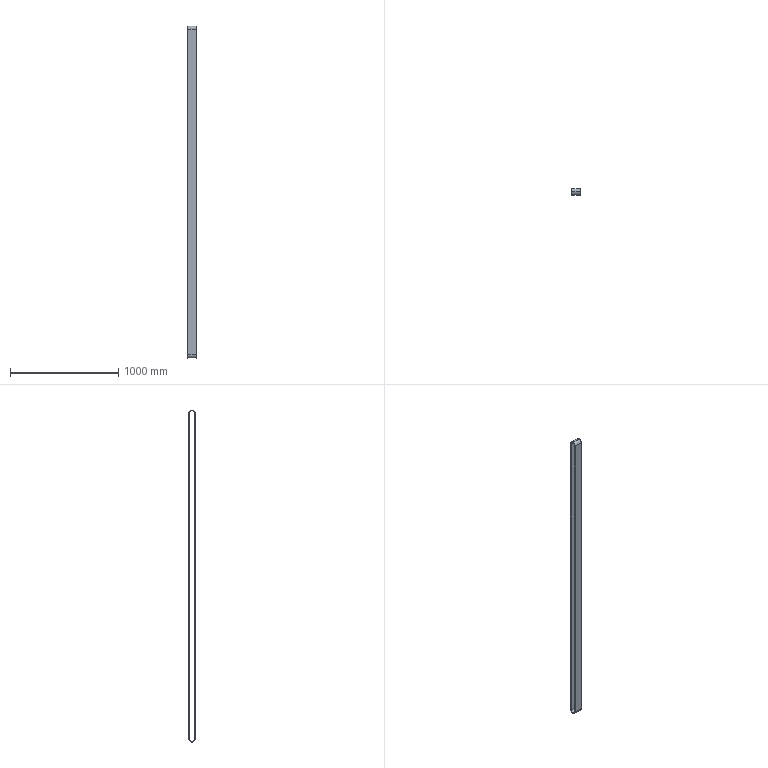Part | SolidWorks | features BossThin 1, ExtruThin 1 | 2 solids | 24 faces | box 80 x 59.15 x 3062 mm | volume 2509466 mm3 | cylinder 12 | plane 12 | commonest cylinder face diameters 54.65 x6 48.99 x3 59.15 x3
STEP:
#1=CARTESIAN_POINT('',(40.,27.325,0.));
#2=VERTEX_POINT('',#1);
#3=CARTESIAN_POINT('',(40.,0.,27.325));
#4=VERTEX_POINT('',#3);
#5=CARTESIAN_POINT('',(40.,0.,0.));
#6=DIRECTION('',(1.,0.,0.));
#7=DIRECTION('',(0.,0.,-1.));
#8=AXIS2_PLACEMENT_3D('',#5,#6,#7);
#9=CIRCLE('',#8,27.325);
#10=EDGE_CURVE('',#2,#4,#9,.T.);
#11=ORIENTED_EDGE('',*,*,#10,.T.);
#12=CARTESIAN_POINT('',(-40.,0.,27.325));
#13=VERTEX_POINT('',#12);
#14=CARTESIAN_POINT('',(40.,0.,27.325));
#15=DIRECTION('',(-1.,0.,0.));
#16=VECTOR('',#15,1000.);
#17=LINE('',#14,#16);
#18=EDGE_CURVE('',#4,#13,#17,.T.);
#19=ORIENTED_EDGE('',*,*,#18,.T.);
#20=CARTESIAN_POINT('',(-40.,27.325,0.));
#21=VERTEX_POINT('',#20);
#22=CARTESIAN_POINT('',(-40.,0.,0.));
#23=DIRECTION('',(1.,0.,0.));
#24=DIRECTION('',(0.,0.,-1.));
#25=AXIS2_PLACEMENT_3D('',#22,#23,#24);
#26=CIRCLE('',#25,27.325);
#27=EDGE_CURVE('',#21,#13,#26,.T.);
#28=ORIENTED_EDGE('',*,*,#27,.F.);
#29=CARTESIAN_POINT('',(40.,27.325,0.));
#30=DIRECTION('',(-1.,0.,0.));
#31=VECTOR('',#30,1000.);
#32=LINE('',#29,#31);
#33=EDGE_CURVE('',#2,#21,#32,.T.);
#34=ORIENTED_EDGE('',*,*,#33,.F.);
#35=EDGE_LOOP('',(#11,#19,#28,#34));
#36=FACE_OUTER_BOUND('',#35,.T.);
#37=CARTESIAN_POINT('',(40.,0.,0.));
#38=DIRECTION('',(-1.,0.,0.));
#39=DIRECTION('',(0.,0.,1.));
#40=AXIS2_PLACEMENT_3D('',#37,#38,#39);
#41=CYLINDRICAL_SURFACE('',#40,27.325);
#42=ADVANCED_FACE('',(#36),#41,.F.);
#43=CARTESIAN_POINT('',(40.,0.,29.575));
#44=VERTEX_POINT('',#43);
#45=CARTESIAN_POINT('',(40.,-29.575,0.));
#46=VERTEX_POINT('',#45);
#47=CARTESIAN_POINT('',(40.,0.,0.));
#48=DIRECTION('',(1.,0.,0.));
#49=DIRECTION('',(0.,0.,-1.));
#50=AXIS2_PLACEMENT_3D('',#47,#48,#49);
#51=CIRCLE('',#50,29.575);
#52=EDGE_CURVE('',#44,#46,#51,.T.);
#53=ORIENTED_EDGE('',*,*,#52,.F.);
#54=CARTESIAN_POINT('',(-40.,0.,29.575));
#55=VERTEX_POINT('',#54);
#56=CARTESIAN_POINT('',(40.,0.,29.575));
#57=DIRECTION('',(-1.,0.,0.));
#58=VECTOR('',#57,1000.);
#59=LINE('',#56,#58);
#60=EDGE_CURVE('',#44,#55,#59,.T.);
#61=ORIENTED_EDGE('',*,*,#60,.T.);
#62=CARTESIAN_POINT('',(-40.,-29.575,0.));
#63=VERTEX_POINT('',#62);
#64=CARTESIAN_POINT('',(-40.,0.,0.));
#65=DIRECTION('',(1.,0.,0.));
#66=DIRECTION('',(0.,0.,-1.));
#67=AXIS2_PLACEMENT_3D('',#64,#65,#66);
#68=CIRCLE('',#67,29.575);
#69=EDGE_CURVE('',#55,#63,#68,.T.);
#70=ORIENTED_EDGE('',*,*,#69,.T.);
#71=CARTESIAN_POINT('',(40.,-29.575,0.));
#72=DIRECTION('',(-1.,0.,0.));
#73=VECTOR('',#72,1000.);
#74=LINE('',#71,#73);
#75=EDGE_CURVE('',#46,#63,#74,.T.);
#76=ORIENTED_EDGE('',*,*,#75,.F.);
#77=EDGE_LOOP('',(#53,#61,#70,#76));
#78=FACE_OUTER_BOUND('',#77,.T.);
#79=CARTESIAN_POINT('',(40.,0.,0.));
#80=DIRECTION('',(-1.,0.,0.));
#81=DIRECTION('',(0.,0.,1.));
#82=AXIS2_PLACEMENT_3D('',#79,#80,#81);
#83=CYLINDRICAL_SURFACE('',#82,29.575);
#84=ADVANCED_FACE('',(#78),#83,.T.);
#85=CARTESIAN_POINT('',(40.,29.575,0.));
#86=VERTEX_POINT('',#85);
#87=CARTESIAN_POINT('',(40.,0.,0.));
#88=DIRECTION('',(1.,0.,0.));
#89=DIRECTION('',(0.,0.,-1.));
#90=AXIS2_PLACEMENT_3D('',#87,#88,#89);
#91=CIRCLE('',#90,29.575);
#92=EDGE_CURVE('',#86,#44,#91,.T.);
#93=ORIENTED_EDGE('',*,*,#92,.T.);
#94=ORIENTED_EDGE('',*,*,#52,.T.);
#95=CARTESIAN_POINT('',(40.,-29.575,-3002.5));
#96=VERTEX_POINT('',#95);
#97=CARTESIAN_POINT('',(40.,-29.575,0.));
#98=DIRECTION('',(0.,0.,-1.));
#99=VECTOR('',#98,1000.);
#100=LINE('',#97,#99);
#101=EDGE_CURVE('',#46,#96,#100,.T.);
#102=ORIENTED_EDGE('',*,*,#101,.T.);
#103=CARTESIAN_POINT('',(40.,29.575,-3002.5));
#104=VERTEX_POINT('',#103);
#105=CARTESIAN_POINT('',(40.,0.,-3002.5));
#106=DIRECTION('',(1.,0.,0.));
#107=DIRECTION('',(0.,0.,-1.));
#108=AXIS2_PLACEMENT_3D('',#105,#106,#107);
#109=CIRCLE('',#108,29.575);
#110=EDGE_CURVE('',#96,#104,#109,.T.);
#111=ORIENTED_EDGE('',*,*,#110,.T.);
#112=CARTESIAN_POINT('',(40.,29.575,0.));
#113=DIRECTION('',(0.,0.,1.));
#114=VECTOR('',#113,1000.);
#115=LINE('',#112,#114);
#116=EDGE_CURVE('',#104,#86,#115,.T.);
#117=ORIENTED_EDGE('',*,*,#116,.T.);
#118=EDGE_LOOP('',(#93,#94,#102,#111,#117));
#119=FACE_OUTER_BOUND('',#118,.T.);
#120=CARTESIAN_POINT('',(40.,-27.325,0.));
#121=VERTEX_POINT('',#120);
#122=CARTESIAN_POINT('',(40.,-27.325,-3002.5));
#123=VERTEX_POINT('',#122);
#124=CARTESIAN_POINT('',(40.,-27.325,0.));
#125=DIRECTION('',(0.,0.,-1.));
#126=VECTOR('',#125,1000.);
#127=LINE('',#124,#126);
#128=EDGE_CURVE('',#121,#123,#127,.T.);
#129=ORIENTED_EDGE('',*,*,#128,.F.);
#130=CARTESIAN_POINT('',(40.,0.,0.));
#131=DIRECTION('',(1.,0.,0.));
#132=DIRECTION('',(0.,0.,-1.));
#133=AXIS2_PLACEMENT_3D('',#130,#131,#132);
#134=CIRCLE('',#133,27.325);
#135=EDGE_CURVE('',#4,#121,#134,.T.);
#136=ORIENTED_EDGE('',*,*,#135,.F.);
#137=ORIENTED_EDGE('',*,*,#10,.F.);
#138=CARTESIAN_POINT('',(40.,27.325,-3002.5));
#139=VERTEX_POINT('',#138);
#140=CARTESIAN_POINT('',(40.,27.325,0.));
#141=DIRECTION('',(0.,0.,1.));
#142=VECTOR('',#141,1000.);
#143=LINE('',#140,#142);
#144=EDGE_CURVE('',#139,#2,#143,.T.);
#145=ORIENTED_EDGE('',*,*,#144,.F.);
#146=CARTESIAN_POINT('',(40.,0.,-3002.5));
#147=DIRECTION('',(1.,0.,0.));
#148=DIRECTION('',(0.,0.,-1.));
#149=AXIS2_PLACEMENT_3D('',#146,#147,#148);
#150=CIRCLE('',#149,27.325);
#151=EDGE_CURVE('',#123,#139,#150,.T.);
#152=ORIENTED_EDGE('',*,*,#151,.F.);
#153=EDGE_LOOP('',(#129,#136,#137,#145,#152));
#154=FACE_BOUND('',#153,.T.);
#155=CARTESIAN_POINT('',(40.,0.,0.));
#156=DIRECTION('',(1.,0.,0.));
#157=DIRECTION('',(0.,0.,-1.));
#158=AXIS2_PLACEMENT_3D('',#155,#156,#157);
#159=PLANE('',#158);
#160=ADVANCED_FACE('',(#119,#154),#159,.T.);
#161=CARTESIAN_POINT('',(-40.,29.575,0.));
#162=VERTEX_POINT('',#161);
#163=CARTESIAN_POINT('',(-40.,0.,0.));
#164=DIRECTION('',(1.,0.,0.));
#165=DIRECTION('',(0.,0.,-1.));
#166=AXIS2_PLACEMENT_3D('',#163,#164,#165);
#167=CIRCLE('',#166,29.575);
#168=EDGE_CURVE('',#162,#55,#167,.T.);
#169=ORIENTED_EDGE('',*,*,#168,.F.);
#170=CARTESIAN_POINT('',(-40.,29.575,-3002.5));
#171=VERTEX_POINT('',#170);
#172=CARTESIAN_POINT('',(-40.,29.575,0.));
#173=DIRECTION('',(0.,0.,1.));
#174=VECTOR('',#173,1000.);
#175=LINE('',#172,#174);
#176=EDGE_CURVE('',#171,#162,#175,.T.);
#177=ORIENTED_EDGE('',*,*,#176,.F.);
#178=CARTESIAN_POINT('',(-40.,-29.575,-3002.5));
#179=VERTEX_POINT('',#178);
#180=CARTESIAN_POINT('',(-40.,0.,-3002.5));
#181=DIRECTION('',(1.,0.,0.));
#182=DIRECTION('',(0.,0.,-1.));
#183=AXIS2_PLACEMENT_3D('',#180,#181,#182);
#184=CIRCLE('',#183,29.575);
#185=EDGE_CURVE('',#179,#171,#184,.T.);
#186=ORIENTED_EDGE('',*,*,#185,.F.);
#187=CARTESIAN_POINT('',(-40.,-29.575,0.));
#188=DIRECTION('',(0.,0.,-1.));
#189=VECTOR('',#188,1000.);
#190=LINE('',#187,#189);
#191=EDGE_CURVE('',#63,#179,#190,.T.);
#192=ORIENTED_EDGE('',*,*,#191,.F.);
#193=ORIENTED_EDGE('',*,*,#69,.F.);
#194=EDGE_LOOP('',(#169,#177,#186,#192,#193));
#195=FACE_OUTER_BOUND('',#194,.T.);
#196=ORIENTED_EDGE('',*,*,#27,.T.);
#197=CARTESIAN_POINT('',(-40.,-27.325,0.));
#198=VERTEX_POINT('',#197);
#199=CARTESIAN_POINT('',(-40.,0.,0.));
#200=DIRECTION('',(1.,0.,0.));
#201=DIRECTION('',(0.,0.,-1.));
#202=AXIS2_PLACEMENT_3D('',#199,#200,#201);
#203=CIRCLE('',#202,27.325);
#204=EDGE_CURVE('',#13,#198,#203,.T.);
#205=ORIENTED_EDGE('',*,*,#204,.T.);
#206=CARTESIAN_POINT('',(-40.,-27.325,-3002.5));
#207=VERTEX_POINT('',#206);
#208=CARTESIAN_POINT('',(-40.,-27.325,0.));
#209=DIRECTION('',(0.,0.,-1.));
#210=VECTOR('',#209,1000.);
#211=LINE('',#208,#210);
#212=EDGE_CURVE('',#198,#207,#211,.T.);
#213=ORIENTED_EDGE('',*,*,#212,.T.);
#214=CARTESIAN_POINT('',(-40.,27.325,-3002.5));
#215=VERTEX_POINT('',#214);
#216=CARTESIAN_POINT('',(-40.,0.,-3002.5));
#217=DIRECTION('',(1.,0.,0.));
#218=DIRECTION('',(0.,0.,-1.));
#219=AXIS2_PLACEMENT_3D('',#216,#217,#218);
#220=CIRCLE('',#219,27.325);
#221=EDGE_CURVE('',#207,#215,#220,.T.);
#222=ORIENTED_EDGE('',*,*,#221,.T.);
#223=CARTESIAN_POINT('',(-40.,27.325,0.));
#224=DIRECTION('',(0.,0.,1.));
#225=VECTOR('',#224,1000.);
#226=LINE('',#223,#225);
#227=EDGE_CURVE('',#215,#21,#226,.T.);
#228=ORIENTED_EDGE('',*,*,#227,.T.);
#229=EDGE_LOOP('',(#196,#205,#213,#222,#228));
#230=FACE_BOUND('',#229,.T.);
#231=CARTESIAN_POINT('',(-40.,0.,0.));
#232=DIRECTION('',(1.,0.,0.));
#233=DIRECTION('',(0.,0.,-1.));
#234=AXIS2_PLACEMENT_3D('',#231,#232,#233);
#235=PLANE('',#234);
#236=ADVANCED_FACE('',(#195,#230),#235,.F.);
#237=ORIENTED_EDGE('',*,*,#60,.F.);
#238=ORIENTED_EDGE('',*,*,#92,.F.);
#239=CARTESIAN_POINT('',(40.,29.575,0.));
#240=DIRECTION('',(-1.,0.,0.));
#241=VECTOR('',#240,1000.);
#242=LINE('',#239,#241);
#243=EDGE_CURVE('',#86,#162,#242,.T.);
#244=ORIENTED_EDGE('',*,*,#243,.T.);
#245=ORIENTED_EDGE('',*,*,#168,.T.);
#246=EDGE_LOOP('',(#237,#238,#244,#245));
#247=FACE_OUTER_BOUND('',#246,.T.);
#248=CARTESIAN_POINT('',(40.,0.,0.));
#249=DIRECTION('',(-1.,0.,0.));
#250=DIRECTION('',(0.,0.,1.));
#251=AXIS2_PLACEMENT_3D('',#248,#249,#250);
#252=CYLINDRICAL_SURFACE('',#251,29.575);
#253=ADVANCED_FACE('',(#247),#252,.T.);
#254=ORIENTED_EDGE('',*,*,#191,.T.);
#255=CARTESIAN_POINT('',(40.,-29.575,-3002.5));
#256=DIRECTION('',(-1.,0.,0.));
#257=VECTOR('',#256,1000.);
#258=LINE('',#255,#257);
#259=EDGE_CURVE('',#96,#179,#258,.T.);
#260=ORIENTED_EDGE('',*,*,#259,.F.);
#261=ORIENTED_EDGE('',*,*,#101,.F.);
#262=ORIENTED_EDGE('',*,*,#75,.T.);
#263=EDGE_LOOP('',(#254,#260,#261,#262));
#264=FACE_OUTER_BOUND('',#263,.T.);
#265=CARTESIAN_POINT('',(40.,-29.575,0.));
#266=DIRECTION('',(0.,1.,0.));
#267=DIRECTION('',(0.,0.,1.));
#268=AXIS2_PLACEMENT_3D('',#265,#266,#267);
#269=PLANE('',#268);
#270=ADVANCED_FACE('',(#264),#269,.F.);
#271=ORIENTED_EDGE('',*,*,#185,.T.);
#272=CARTESIAN_POINT('',(40.,29.575,-3002.5));
#273=DIRECTION('',(-1.,0.,0.));
#274=VECTOR('',#273,1000.);
#275=LINE('',#272,#274);
#276=EDGE_CURVE('',#104,#171,#275,.T.);
#277=ORIENTED_EDGE('',*,*,#276,.F.);
#278=ORIENTED_EDGE('',*,*,#110,.F.);
#279=ORIENTED_EDGE('',*,*,#259,.T.);
#280=EDGE_LOOP('',(#271,#277,#278,#279));
#281=FACE_OUTER_BOUND('',#280,.T.);
#282=CARTESIAN_POINT('',(40.,0.,-3002.5));
#283=DIRECTION('',(-1.,0.,0.));
#284=DIRECTION('',(0.,0.,1.));
#285=AXIS2_PLACEMENT_3D('',#282,#283,#284);
#286=CYLINDRICAL_SURFACE('',#285,29.575);
#287=ADVANCED_FACE('',(#281),#286,.T.);
#288=ORIENTED_EDGE('',*,*,#176,.T.);
#289=ORIENTED_EDGE('',*,*,#243,.F.);
#290=ORIENTED_EDGE('',*,*,#116,.F.);
#291=ORIENTED_EDGE('',*,*,#276,.T.);
#292=EDGE_LOOP('',(#288,#289,#290,#291));
#293=FACE_OUTER_BOUND('',#292,.T.);
#294=CARTESIAN_POINT('',(40.,29.575,0.));
#295=DIRECTION('',(0.,-1.,0.));
#296=DIRECTION('',(0.,0.,-1.));
#297=AXIS2_PLACEMENT_3D('',#294,#295,#296);
#298=PLANE('',#297);
#299=ADVANCED_FACE('',(#293),#298,.F.);
#300=ORIENTED_EDGE('',*,*,#18,.F.);
#301=ORIENTED_EDGE('',*,*,#135,.T.);
#302=CARTESIAN_POINT('',(40.,-27.325,0.));
#303=DIRECTION('',(-1.,0.,0.));
#304=VECTOR('',#303,1000.);
#305=LINE('',#302,#304);
#306=EDGE_CURVE('',#121,#198,#305,.T.);
#307=ORIENTED_EDGE('',*,*,#306,.T.);
#308=ORIENTED_EDGE('',*,*,#204,.F.);
#309=EDGE_LOOP('',(#300,#301,#307,#308));
#310=FACE_OUTER_BOUND('',#309,.T.);
#311=CARTESIAN_POINT('',(40.,0.,0.));
#312=DIRECTION('',(-1.,0.,0.));
#313=DIRECTION('',(0.,0.,1.));
#314=AXIS2_PLACEMENT_3D('',#311,#312,#313);
#315=CYLINDRICAL_SURFACE('',#314,27.325);
#316=ADVANCED_FACE('',(#310),#315,.F.);
#317=ORIENTED_EDGE('',*,*,#212,.F.);
#318=ORIENTED_EDGE('',*,*,#306,.F.);
#319=ORIENTED_EDGE('',*,*,#128,.T.);
#320=CARTESIAN_POINT('',(40.,-27.325,-3002.5));
#321=DIRECTION('',(-1.,0.,0.));
#322=VECTOR('',#321,1000.);
#323=LINE('',#320,#322);
#324=EDGE_CURVE('',#123,#207,#323,.T.);
#325=ORIENTED_EDGE('',*,*,#324,.T.);
#326=EDGE_LOOP('',(#317,#318,#319,#325));
#327=FACE_OUTER_BOUND('',#326,.T.);
#328=CARTESIAN_POINT('',(40.,-27.325,0.));
#329=DIRECTION('',(0.,1.,0.));
#330=DIRECTION('',(0.,0.,1.));
#331=AXIS2_PLACEMENT_3D('',#328,#329,#330);
#332=PLANE('',#331);
#333=ADVANCED_FACE('',(#327),#332,.T.);
#334=ORIENTED_EDGE('',*,*,#221,.F.);
#335=ORIENTED_EDGE('',*,*,#324,.F.);
#336=ORIENTED_EDGE('',*,*,#151,.T.);
#337=CARTESIAN_POINT('',(40.,27.325,-3002.5));
#338=DIRECTION('',(-1.,0.,0.));
#339=VECTOR('',#338,1000.);
#340=LINE('',#337,#339);
#341=EDGE_CURVE('',#139,#215,#340,.T.);
#342=ORIENTED_EDGE('',*,*,#341,.T.);
#343=EDGE_LOOP('',(#334,#335,#336,#342));
#344=FACE_OUTER_BOUND('',#343,.T.);
#345=CARTESIAN_POINT('',(40.,0.,-3002.5));
#346=DIRECTION('',(-1.,0.,0.));
#347=DIRECTION('',(0.,0.,1.));
#348=AXIS2_PLACEMENT_3D('',#345,#346,#347);
#349=CYLINDRICAL_SURFACE('',#348,27.325);
#350=ADVANCED_FACE('',(#344),#349,.F.);
#351=ORIENTED_EDGE('',*,*,#227,.F.);
#352=ORIENTED_EDGE('',*,*,#341,.F.);
#353=ORIENTED_EDGE('',*,*,#144,.T.);
#354=ORIENTED_EDGE('',*,*,#33,.T.);
#355=EDGE_LOOP('',(#351,#352,#353,#354));
#356=FACE_OUTER_BOUND('',#355,.T.);
#357=CARTESIAN_POINT('',(40.,27.325,0.));
#358=DIRECTION('',(0.,-1.,0.));
#359=DIRECTION('',(0.,0.,-1.));
#360=AXIS2_PLACEMENT_3D('',#357,#358,#359);
#361=PLANE('',#360);
#362=ADVANCED_FACE('',(#356),#361,.T.);
#363=CLOSED_SHELL('',(#42,#84,#160,#236,#253,#270,#287,#299,#316,#333,#350,#362));
#364=MANIFOLD_SOLID_BREP('',#363);
#365=CARTESIAN_POINT('',(40.,24.495,0.));
#366=VERTEX_POINT('',#365);
#367=CARTESIAN_POINT('',(40.,0.,24.495));
#368=VERTEX_POINT('',#367);
#369=CARTESIAN_POINT('',(40.,0.,0.));
#370=DIRECTION('',(1.,0.,0.));
#371=DIRECTION('',(0.,0.,-1.));
#372=AXIS2_PLACEMENT_3D('',#369,#370,#371);
#373=CIRCLE('',#372,24.495);
#374=EDGE_CURVE('',#366,#368,#373,.T.);
#375=ORIENTED_EDGE('',*,*,#374,.T.);
#376=CARTESIAN_POINT('',(-40.,0.,24.495));
#377=VERTEX_POINT('',#376);
#378=CARTESIAN_POINT('',(40.,0.,24.495));
#379=DIRECTION('',(-1.,0.,0.));
#380=VECTOR('',#379,1000.);
#381=LINE('',#378,#380);
#382=EDGE_CURVE('',#368,#377,#381,.T.);
#383=ORIENTED_EDGE('',*,*,#382,.T.);
#384=CARTESIAN_POINT('',(-40.,24.495,0.));
#385=VERTEX_POINT('',#384);
#386=CARTESIAN_POINT('',(-40.,0.,0.));
#387=DIRECTION('',(1.,0.,0.));
#388=DIRECTION('',(0.,0.,-1.));
#389=AXIS2_PLACEMENT_3D('',#386,#387,#388);
#390=CIRCLE('',#389,24.495);
#391=EDGE_CURVE('',#385,#377,#390,.T.);
#392=ORIENTED_EDGE('',*,*,#391,.F.);
#393=CARTESIAN_POINT('',(40.,24.495,0.));
#394=DIRECTION('',(-1.,0.,0.));
#395=VECTOR('',#394,1000.);
#396=LINE('',#393,#395);
#397=EDGE_CURVE('',#366,#385,#396,.T.);
#398=ORIENTED_EDGE('',*,*,#397,.F.);
#399=EDGE_LOOP('',(#375,#383,#392,#398));
#400=FACE_OUTER_BOUND('',#399,.T.);
#401=CARTESIAN_POINT('',(40.,0.,0.));
#402=DIRECTION('',(-1.,0.,0.));
#403=DIRECTION('',(0.,0.,1.));
#404=AXIS2_PLACEMENT_3D('',#401,#402,#403);
#405=CYLINDRICAL_SURFACE('',#404,24.495);
#406=ADVANCED_FACE('',(#400),#405,.F.);
#407=CARTESIAN_POINT('',(40.,0.,27.325));
#408=VERTEX_POINT('',#407);
#409=CARTESIAN_POINT('',(40.,-27.325,0.));
#410=VERTEX_POINT('',#409);
#411=CARTESIAN_POINT('',(40.,0.,0.));
#412=DIRECTION('',(1.,0.,0.));
#413=DIRECTION('',(0.,0.,-1.));
#414=AXIS2_PLACEMENT_3D('',#411,#412,#413);
#415=CIRCLE('',#414,27.325);
#416=EDGE_CURVE('',#408,#410,#415,.T.);
#417=ORIENTED_EDGE('',*,*,#416,.F.);
#418=CARTESIAN_POINT('',(-40.,0.,27.325));
#419=VERTEX_POINT('',#418);
#420=CARTESIAN_POINT('',(40.,0.,27.325));
#421=DIRECTION('',(-1.,0.,0.));
#422=VECTOR('',#421,1000.);
#423=LINE('',#420,#422);
#424=EDGE_CURVE('',#408,#419,#423,.T.);
#425=ORIENTED_EDGE('',*,*,#424,.T.);
#426=CARTESIAN_POINT('',(-40.,-27.325,0.));
#427=VERTEX_POINT('',#426);
#428=CARTESIAN_POINT('',(-40.,0.,0.));
#429=DIRECTION('',(1.,0.,0.));
#430=DIRECTION('',(0.,0.,-1.));
#431=AXIS2_PLACEMENT_3D('',#428,#429,#430);
#432=CIRCLE('',#431,27.325);
#433=EDGE_CURVE('',#419,#427,#432,.T.);
#434=ORIENTED_EDGE('',*,*,#433,.T.);
#435=CARTESIAN_POINT('',(40.,-27.325,0.));
#436=DIRECTION('',(-1.,0.,0.));
#437=VECTOR('',#436,1000.);
#438=LINE('',#435,#437);
#439=EDGE_CURVE('',#410,#427,#438,.T.);
#440=ORIENTED_EDGE('',*,*,#439,.F.);
#441=EDGE_LOOP('',(#417,#425,#434,#440));
#442=FACE_OUTER_BOUND('',#441,.T.);
#443=CARTESIAN_POINT('',(40.,0.,0.));
#444=DIRECTION('',(-1.,0.,0.));
#445=DIRECTION('',(0.,0.,1.));
#446=AXIS2_PLACEMENT_3D('',#443,#444,#445);
#447=CYLINDRICAL_SURFACE('',#446,27.325);
#448=ADVANCED_FACE('',(#442),#447,.T.);
#449=CARTESIAN_POINT('',(40.,27.325,0.));
#450=VERTEX_POINT('',#449);
#451=CARTESIAN_POINT('',(40.,0.,0.));
#452=DIRECTION('',(1.,0.,0.));
#453=DIRECTION('',(0.,0.,-1.));
#454=AXIS2_PLACEMENT_3D('',#451,#452,#453);
#455=CIRCLE('',#454,27.325);
#456=EDGE_CURVE('',#450,#408,#455,.T.);
#457=ORIENTED_EDGE('',*,*,#456,.T.);
#458=ORIENTED_EDGE('',*,*,#416,.T.);
#459=CARTESIAN_POINT('',(40.,-27.325,-3002.5));
#460=VERTEX_POINT('',#459);
#461=CARTESIAN_POINT('',(40.,-27.325,0.));
#462=DIRECTION('',(0.,0.,-1.));
#463=VECTOR('',#462,1000.);
#464=LINE('',#461,#463);
#465=EDGE_CURVE('',#410,#460,#464,.T.);
#466=ORIENTED_EDGE('',*,*,#465,.T.);
#467=CARTESIAN_POINT('',(40.,27.325,-3002.5));
#468=VERTEX_POINT('',#467);
#469=CARTESIAN_POINT('',(40.,0.,-3002.5));
#470=DIRECTION('',(1.,0.,0.));
#471=DIRECTION('',(0.,0.,-1.));
#472=AXIS2_PLACEMENT_3D('',#469,#470,#471);
#473=CIRCLE('',#472,27.325);
#474=EDGE_CURVE('',#460,#468,#473,.T.);
#475=ORIENTED_EDGE('',*,*,#474,.T.);
#476=CARTESIAN_POINT('',(40.,27.325,-3002.5));
#477=DIRECTION('',(0.,0.,1.));
#478=VECTOR('',#477,1000.);
#479=LINE('',#476,#478);
#480=EDGE_CURVE('',#468,#450,#479,.T.);
#481=ORIENTED_EDGE('',*,*,#480,.T.);
#482=EDGE_LOOP('',(#457,#458,#466,#475,#481));
#483=FACE_OUTER_BOUND('',#482,.T.);
#484=CARTESIAN_POINT('',(40.,-24.495,0.));
#485=VERTEX_POINT('',#484);
#486=CARTESIAN_POINT('',(40.,-24.495,-3002.5));
#487=VERTEX_POINT('',#486);
#488=CARTESIAN_POINT('',(40.,-24.495,0.));
#489=DIRECTION('',(0.,0.,-1.));
#490=VECTOR('',#489,1000.);
#491=LINE('',#488,#490);
#492=EDGE_CURVE('',#485,#487,#491,.T.);
#493=ORIENTED_EDGE('',*,*,#492,.F.);
#494=CARTESIAN_POINT('',(40.,0.,0.));
#495=DIRECTION('',(1.,0.,0.));
#496=DIRECTION('',(0.,0.,-1.));
#497=AXIS2_PLACEMENT_3D('',#494,#495,#496);
#498=CIRCLE('',#497,24.495);
#499=EDGE_CURVE('',#368,#485,#498,.T.);
#500=ORIENTED_EDGE('',*,*,#499,.F.);
#501=ORIENTED_EDGE('',*,*,#374,.F.);
#502=CARTESIAN_POINT('',(40.,24.495,-3002.5));
#503=VERTEX_POINT('',#502);
#504=CARTESIAN_POINT('',(40.,24.495,-3002.5));
#505=DIRECTION('',(0.,0.,1.));
#506=VECTOR('',#505,1000.);
#507=LINE('',#504,#506);
#508=EDGE_CURVE('',#503,#366,#507,.T.);
#509=ORIENTED_EDGE('',*,*,#508,.F.);
#510=CARTESIAN_POINT('',(40.,0.,-3002.5));
#511=DIRECTION('',(1.,0.,0.));
#512=DIRECTION('',(0.,0.,-1.));
#513=AXIS2_PLACEMENT_3D('',#510,#511,#512);
#514=CIRCLE('',#513,24.495);
#515=EDGE_CURVE('',#487,#503,#514,.T.);
#516=ORIENTED_EDGE('',*,*,#515,.F.);
#517=EDGE_LOOP('',(#493,#500,#501,#509,#516));
#518=FACE_BOUND('',#517,.T.);
#519=CARTESIAN_POINT('',(40.,0.,0.));
#520=DIRECTION('',(1.,0.,0.));
#521=DIRECTION('',(0.,0.,-1.));
#522=AXIS2_PLACEMENT_3D('',#519,#520,#521);
#523=PLANE('',#522);
#524=ADVANCED_FACE('',(#483,#518),#523,.T.);
#525=CARTESIAN_POINT('',(-40.,27.325,0.));
#526=VERTEX_POINT('',#525);
#527=CARTESIAN_POINT('',(-40.,0.,0.));
#528=DIRECTION('',(1.,0.,0.));
#529=DIRECTION('',(0.,0.,-1.));
#530=AXIS2_PLACEMENT_3D('',#527,#528,#529);
#531=CIRCLE('',#530,27.325);
#532=EDGE_CURVE('',#526,#419,#531,.T.);
#533=ORIENTED_EDGE('',*,*,#532,.F.);
#534=CARTESIAN_POINT('',(-40.,27.325,-3002.5));
#535=VERTEX_POINT('',#534);
#536=CARTESIAN_POINT('',(-40.,27.325,-3002.5));
#537=DIRECTION('',(0.,0.,1.));
#538=VECTOR('',#537,1000.);
#539=LINE('',#536,#538);
#540=EDGE_CURVE('',#535,#526,#539,.T.);
#541=ORIENTED_EDGE('',*,*,#540,.F.);
#542=CARTESIAN_POINT('',(-40.,-27.325,-3002.5));
#543=VERTEX_POINT('',#542);
#544=CARTESIAN_POINT('',(-40.,0.,-3002.5));
#545=DIRECTION('',(1.,0.,0.));
#546=DIRECTION('',(0.,0.,-1.));
#547=AXIS2_PLACEMENT_3D('',#544,#545,#546);
#548=CIRCLE('',#547,27.325);
#549=EDGE_CURVE('',#543,#535,#548,.T.);
#550=ORIENTED_EDGE('',*,*,#549,.F.);
#551=CARTESIAN_POINT('',(-40.,-27.325,0.));
#552=DIRECTION('',(0.,0.,-1.));
#553=VECTOR('',#552,1000.);
#554=LINE('',#551,#553);
#555=EDGE_CURVE('',#427,#543,#554,.T.);
#556=ORIENTED_EDGE('',*,*,#555,.F.);
#557=ORIENTED_EDGE('',*,*,#433,.F.);
#558=EDGE_LOOP('',(#533,#541,#550,#556,#557));
#559=FACE_OUTER_BOUND('',#558,.T.);
#560=ORIENTED_EDGE('',*,*,#391,.T.);
#561=CARTESIAN_POINT('',(-40.,-24.495,0.));
#562=VERTEX_POINT('',#561);
#563=CARTESIAN_POINT('',(-40.,0.,0.));
#564=DIRECTION('',(1.,0.,0.));
#565=DIRECTION('',(0.,0.,-1.));
#566=AXIS2_PLACEMENT_3D('',#563,#564,#565);
#567=CIRCLE('',#566,24.495);
#568=EDGE_CURVE('',#377,#562,#567,.T.);
#569=ORIENTED_EDGE('',*,*,#568,.T.);
#570=CARTESIAN_POINT('',(-40.,-24.495,-3002.5));
#571=VERTEX_POINT('',#570);
#572=CARTESIAN_POINT('',(-40.,-24.495,0.));
#573=DIRECTION('',(0.,0.,-1.));
#574=VECTOR('',#573,1000.);
#575=LINE('',#572,#574);
#576=EDGE_CURVE('',#562,#571,#575,.T.);
#577=ORIENTED_EDGE('',*,*,#576,.T.);
#578=CARTESIAN_POINT('',(-40.,24.495,-3002.5));
#579=VERTEX_POINT('',#578);
#580=CARTESIAN_POINT('',(-40.,0.,-3002.5));
#581=DIRECTION('',(1.,0.,0.));
#582=DIRECTION('',(0.,0.,-1.));
#583=AXIS2_PLACEMENT_3D('',#580,#581,#582);
#584=CIRCLE('',#583,24.495);
#585=EDGE_CURVE('',#571,#579,#584,.T.);
#586=ORIENTED_EDGE('',*,*,#585,.T.);
#587=CARTESIAN_POINT('',(-40.,24.495,-3002.5));
#588=DIRECTION('',(0.,0.,1.));
#589=VECTOR('',#588,1000.);
#590=LINE('',#587,#589);
#591=EDGE_CURVE('',#579,#385,#590,.T.);
#592=ORIENTED_EDGE('',*,*,#591,.T.);
#593=EDGE_LOOP('',(#560,#569,#577,#586,#592));
#594=FACE_BOUND('',#593,.T.);
#595=CARTESIAN_POINT('',(-40.,0.,0.));
#596=DIRECTION('',(1.,0.,0.));
#597=DIRECTION('',(0.,0.,-1.));
#598=AXIS2_PLACEMENT_3D('',#595,#596,#597);
#599=PLANE('',#598);
#600=ADVANCED_FACE('',(#559,#594),#599,.F.);
#601=ORIENTED_EDGE('',*,*,#424,.F.);
#602=ORIENTED_EDGE('',*,*,#456,.F.);
#603=CARTESIAN_POINT('',(40.,27.325,0.));
#604=DIRECTION('',(-1.,0.,0.));
#605=VECTOR('',#604,1000.);
#606=LINE('',#603,#605);
#607=EDGE_CURVE('',#450,#526,#606,.T.);
#608=ORIENTED_EDGE('',*,*,#607,.T.);
#609=ORIENTED_EDGE('',*,*,#532,.T.);
#610=EDGE_LOOP('',(#601,#602,#608,#609));
#611=FACE_OUTER_BOUND('',#610,.T.);
#612=CARTESIAN_POINT('',(40.,0.,0.));
#613=DIRECTION('',(-1.,0.,0.));
#614=DIRECTION('',(0.,0.,1.));
#615=AXIS2_PLACEMENT_3D('',#612,#613,#614);
#616=CYLINDRICAL_SURFACE('',#615,27.325);
#617=ADVANCED_FACE('',(#611),#616,.T.);
#618=ORIENTED_EDGE('',*,*,#555,.T.);
#619=CARTESIAN_POINT('',(40.,-27.325,-3002.5));
#620=DIRECTION('',(-1.,0.,0.));
#621=VECTOR('',#620,1000.);
#622=LINE('',#619,#621);
#623=EDGE_CURVE('',#460,#543,#622,.T.);
#624=ORIENTED_EDGE('',*,*,#623,.F.);
#625=ORIENTED_EDGE('',*,*,#465,.F.);
#626=ORIENTED_EDGE('',*,*,#439,.T.);
#627=EDGE_LOOP('',(#618,#624,#625,#626));
#628=FACE_OUTER_BOUND('',#627,.T.);
#629=CARTESIAN_POINT('',(40.,-27.325,0.));
#630=DIRECTION('',(0.,1.,0.));
#631=DIRECTION('',(0.,0.,1.));
#632=AXIS2_PLACEMENT_3D('',#629,#630,#631);
#633=PLANE('',#632);
#634=ADVANCED_FACE('',(#628),#633,.F.);
#635=ORIENTED_EDGE('',*,*,#549,.T.);
#636=CARTESIAN_POINT('',(40.,27.325,-3002.5));
#637=DIRECTION('',(-1.,0.,0.));
#638=VECTOR('',#637,1000.);
#639=LINE('',#636,#638);
#640=EDGE_CURVE('',#468,#535,#639,.T.);
#641=ORIENTED_EDGE('',*,*,#640,.F.);
#642=ORIENTED_EDGE('',*,*,#474,.F.);
#643=ORIENTED_EDGE('',*,*,#623,.T.);
#644=EDGE_LOOP('',(#635,#641,#642,#643));
#645=FACE_OUTER_BOUND('',#644,.T.);
#646=CARTESIAN_POINT('',(40.,0.,-3002.5));
#647=DIRECTION('',(-1.,0.,0.));
#648=DIRECTION('',(0.,0.,1.));
#649=AXIS2_PLACEMENT_3D('',#646,#647,#648);
#650=CYLINDRICAL_SURFACE('',#649,27.325);
#651=ADVANCED_FACE('',(#645),#650,.T.);
#652=ORIENTED_EDGE('',*,*,#540,.T.);
#653=ORIENTED_EDGE('',*,*,#607,.F.);
#654=ORIENTED_EDGE('',*,*,#480,.F.);
#655=ORIENTED_EDGE('',*,*,#640,.T.);
#656=EDGE_LOOP('',(#652,#653,#654,#655));
#657=FACE_OUTER_BOUND('',#656,.T.);
#658=CARTESIAN_POINT('',(40.,27.325,-3002.5));
#659=DIRECTION('',(0.,-1.,0.));
#660=DIRECTION('',(0.,0.,-1.));
#661=AXIS2_PLACEMENT_3D('',#658,#659,#660);
#662=PLANE('',#661);
#663=ADVANCED_FACE('',(#657),#662,.F.);
#664=ORIENTED_EDGE('',*,*,#382,.F.);
#665=ORIENTED_EDGE('',*,*,#499,.T.);
#666=CARTESIAN_POINT('',(40.,-24.495,0.));
#667=DIRECTION('',(-1.,0.,0.));
#668=VECTOR('',#667,1000.);
#669=LINE('',#666,#668);
#670=EDGE_CURVE('',#485,#562,#669,.T.);
#671=ORIENTED_EDGE('',*,*,#670,.T.);
#672=ORIENTED_EDGE('',*,*,#568,.F.);
#673=EDGE_LOOP('',(#664,#665,#671,#672));
#674=FACE_OUTER_BOUND('',#673,.T.);
#675=CARTESIAN_POINT('',(40.,0.,0.));
#676=DIRECTION('',(-1.,0.,0.));
#677=DIRECTION('',(0.,0.,1.));
#678=AXIS2_PLACEMENT_3D('',#675,#676,#677);
#679=CYLINDRICAL_SURFACE('',#678,24.495);
#680=ADVANCED_FACE('',(#674),#679,.F.);
#681=ORIENTED_EDGE('',*,*,#576,.F.);
#682=ORIENTED_EDGE('',*,*,#670,.F.);
#683=ORIENTED_EDGE('',*,*,#492,.T.);
#684=CARTESIAN_POINT('',(40.,-24.495,-3002.5));
#685=DIRECTION('',(-1.,0.,0.));
#686=VECTOR('',#685,1000.);
#687=LINE('',#684,#686);
#688=EDGE_CURVE('',#487,#571,#687,.T.);
#689=ORIENTED_EDGE('',*,*,#688,.T.);
#690=EDGE_LOOP('',(#681,#682,#683,#689));
#691=FACE_OUTER_BOUND('',#690,.T.);
#692=CARTESIAN_POINT('',(40.,-24.495,0.));
#693=DIRECTION('',(0.,1.,0.));
#694=DIRECTION('',(0.,0.,1.));
#695=AXIS2_PLACEMENT_3D('',#692,#693,#694);
#696=PLANE('',#695);
#697=ADVANCED_FACE('',(#691),#696,.T.);
#698=ORIENTED_EDGE('',*,*,#585,.F.);
#699=ORIENTED_EDGE('',*,*,#688,.F.);
#700=ORIENTED_EDGE('',*,*,#515,.T.);
#701=CARTESIAN_POINT('',(40.,24.495,-3002.5));
#702=DIRECTION('',(-1.,0.,0.));
#703=VECTOR('',#702,1000.);
#704=LINE('',#701,#703);
#705=EDGE_CURVE('',#503,#579,#704,.T.);
#706=ORIENTED_EDGE('',*,*,#705,.T.);
#707=EDGE_LOOP('',(#698,#699,#700,#706));
#708=FACE_OUTER_BOUND('',#707,.T.);
#709=CARTESIAN_POINT('',(40.,0.,-3002.5));
#710=DIRECTION('',(-1.,0.,0.));
#711=DIRECTION('',(0.,0.,1.));
#712=AXIS2_PLACEMENT_3D('',#709,#710,#711);
#713=CYLINDRICAL_SURFACE('',#712,24.495);
#714=ADVANCED_FACE('',(#708),#713,.F.);
#715=ORIENTED_EDGE('',*,*,#591,.F.);
#716=ORIENTED_EDGE('',*,*,#705,.F.);
#717=ORIENTED_EDGE('',*,*,#508,.T.);
#718=ORIENTED_EDGE('',*,*,#397,.T.);
#719=EDGE_LOOP('',(#715,#716,#717,#718));
#720=FACE_OUTER_BOUND('',#719,.T.);
#721=CARTESIAN_POINT('',(40.,24.495,-3002.5));
#722=DIRECTION('',(0.,-1.,0.));
#723=DIRECTION('',(0.,0.,-1.));
#724=AXIS2_PLACEMENT_3D('',#721,#722,#723);
#725=PLANE('',#724);
#726=ADVANCED_FACE('',(#720),#725,.T.);
#727=CLOSED_SHELL('',(#406,#448,#524,#600,#617,#634,#651,#663,#680,#697,#714,#726));
#728=MANIFOLD_SOLID_BREP('',#727);
#729=CARTESIAN_POINT('',(0.,0.,0.));
#730=DIRECTION('',(0.,0.,1.));
#731=DIRECTION('',(1.,0.,0.));
#732=AXIS2_PLACEMENT_3D('',#729,#730,#731);
#733=(LENGTH_UNIT()NAMED_UNIT(*)SI_UNIT(.MILLI.,.METRE.));
#734=UNCERTAINTY_MEASURE_WITH_UNIT(LENGTH_MEASURE(0.00001),#733,'','');
#735=(NAMED_UNIT(*)PLANE_ANGLE_UNIT()SI_UNIT($,.RADIAN.));
#736=(NAMED_UNIT(*)SI_UNIT($,.STERADIAN.)SOLID_ANGLE_UNIT());
#737=(GEOMETRIC_REPRESENTATION_CONTEXT(3)GLOBAL_UNCERTAINTY_ASSIGNED_CONTEXT((#734))GLOBAL_UNIT_ASSIGNED_CONTEXT((#733,#735,#736))REPRESENTATION_CONTEXT('',''));
#738=ADVANCED_BREP_SHAPE_REPRESENTATION('',(#364,#728,#732),#737);